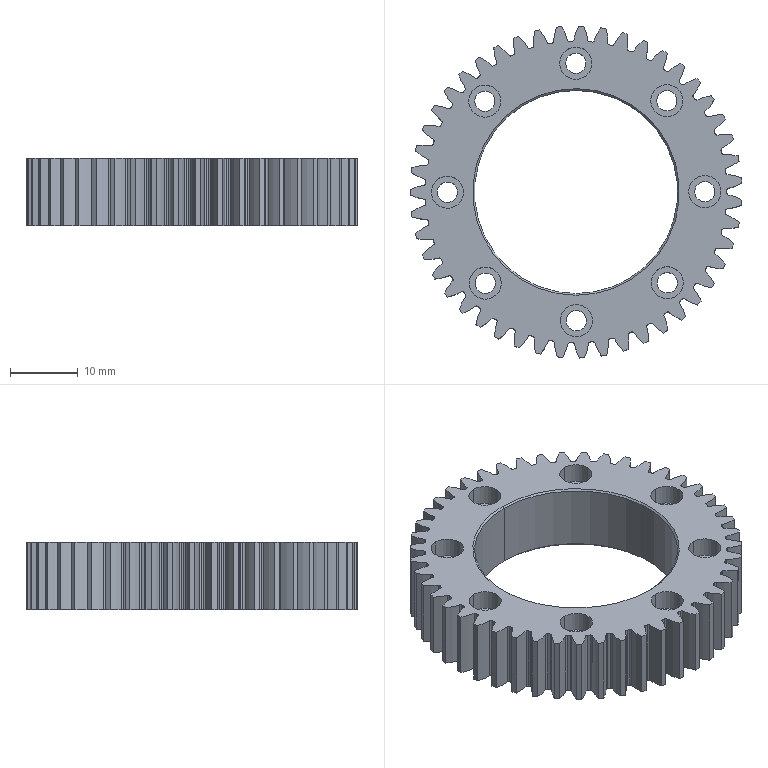Part | STEP file | GEAR_1_BODY-2 | 1 solid | 331 faces | box 48.971 x 48.992 x 10 mm | volume 9344 mm3 | spline 235 | cylinder 82 | plane 10 | cone 4 | commonest cylinder face diameters 44.5 x48 3 x16 4.75 x16 30 x2